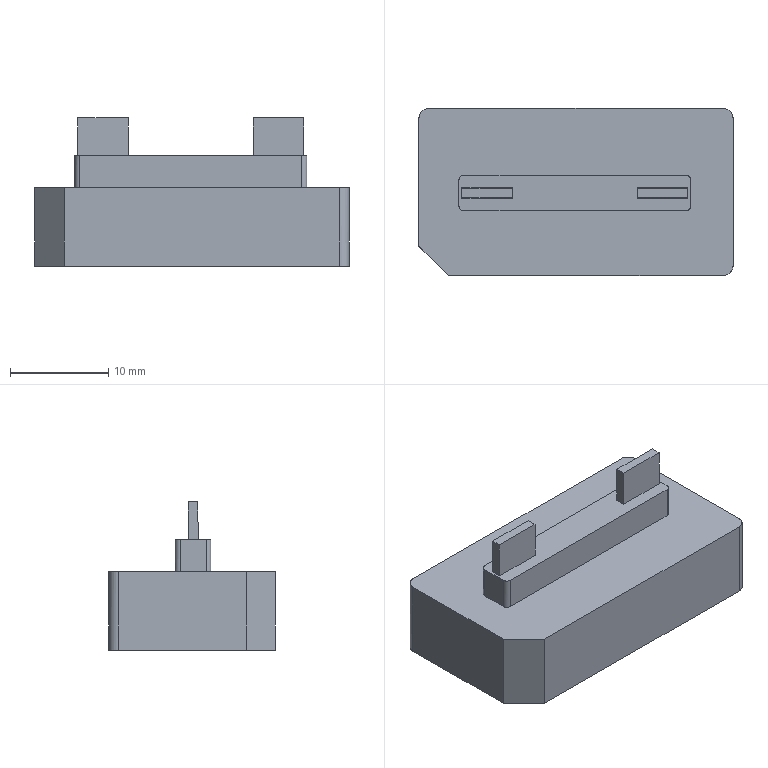NC program | PowerMill | posted by the shop | part box 32 x 17 x 15.109 mm
Lines 3996 to 5578 of 56729:
( TOOL ID   D3_1_1 )
( TOOL DIA. 3. TIP RAD 0 LENGTH 62.28 )
( Z = -7.28 )
T10 M6
T13
G91 G28 Z0
G0 G90 G54
M08
S18000 M3
X0 Y0 M8
G43 Z10.799 H10
X12.158 Y-2.407
Z.922
G1 Z-.278 F1200
X12.15 Y-2.364 F2000
X12.138 Y-2.322
X12.122 Y-2.282
X12.102 Y-2.242
X12.08 Y-2.205
X12.053 Y-2.17
X12.024 Y-2.137
X11.992 Y-2.108
X11.957 Y-2.081
X11.92 Y-2.058
X11.881 Y-2.038
X11.841 Y-2.022
X11.799 Y-2.009
X11.756 Y-2.
X11.712 Y-1.996
X11.669 Y-1.995
X11.625 Y-1.998
X11.615 Y-1.999
X11.542 Y-2.01
X11.471 Y-2.016
X11.402 Y-2.018
X11.333
X8.245
X6.298 Y-2.019
X6.211 Y-2.017
X6.129 Y-2.012
X6.053 Y-2.004
X5.981 Y-1.992
X5.913 Y-1.977
X5.847 Y-1.958
X5.775 Y-1.935
X5.704 Y-1.907
X5.635 Y-1.876
X5.568 Y-1.841
X5.503 Y-1.802
X5.439 Y-1.761
X5.379 Y-1.716
X5.321 Y-1.668
X5.266 Y-1.618
X5.214 Y-1.564
X5.164 Y-1.508
X5.117 Y-1.449
X5.073 Y-1.387
X5.033 Y-1.323
X4.996 Y-1.257
X4.962 Y-1.189
X4.932 Y-1.12
X4.906 Y-1.049
X4.884 Y-.978
X4.866 Y-.905
X4.851 Y-.831
X4.841 Y-.757
X4.834 Y-.683
X4.832 Y-.608
Y-.533
X4.831 Y.3
X4.832 Y.366
X4.834 Y.432
X4.839 Y.498
X4.846 Y.564
X4.856 Y.631
X4.87 Y.699
X4.888 Y.767
X4.91 Y.835
X4.935 Y.9
X4.962 Y.963
X4.992 Y1.026
X5.026 Y1.088
X5.063 Y1.149
X5.105 Y1.21
X5.152 Y1.269
X5.199 Y1.324
X5.25 Y1.378
X5.304 Y1.429
X5.361 Y1.478
X5.421 Y1.524
X5.484 Y1.566
X5.548 Y1.606
X5.615 Y1.642
X5.684 Y1.674
X5.751 Y1.702
X5.821 Y1.726
X5.894 Y1.747
X5.969 Y1.765
X6.034 Y1.777
X6.102 Y1.786
X6.176 Y1.792
X6.26 Y1.794
X6.36 Y1.795
X10.154 Y1.794
X11.397
X11.468 Y1.792
X11.539 Y1.786
X11.61 Y1.777
X11.681 Y1.763
X11.753 Y1.746
X11.825 Y1.724
X11.894 Y1.699
X11.963 Y1.671
X12.031 Y1.638
X12.097 Y1.602
X12.161 Y1.563
X12.223 Y1.52
X12.283 Y1.474
X12.34 Y1.425
X12.395 Y1.372
X12.446 Y1.317
X12.495 Y1.26
X12.541 Y1.2
X12.583 Y1.137
X12.621 Y1.075
X12.656 Y1.009
X12.688 Y.941
X12.716 Y.872
X12.74 Y.803
X12.757 Y.744
X12.772 Y.684
X12.784 Y.624
X12.794 Y.559
X12.802 Y.487
X12.807 Y.407
X12.808 Y.333
X12.809 Y.264
Y.2
X12.808 Y-.397
X12.807 Y-.6
X12.805 Y-.673
X12.799 Y-.747
X12.789 Y-.821
X12.775 Y-.894
X12.758 Y-.967
X12.736 Y-1.04
X12.71 Y-1.111
X12.681 Y-1.18
X12.649 Y-1.248
X12.612 Y-1.313
X12.573 Y-1.377
X12.529 Y-1.439
X12.483 Y-1.499
X12.434 Y-1.555
X12.382 Y-1.61
X12.326 Y-1.661
X12.269 Y-1.709
X12.209 Y-1.754
X12.146 Y-1.796
X12.081 Y-1.835
X12.014 Y-1.871
X11.946 Y-1.902
X11.875 Y-1.93
X11.804 Y-1.955
X11.731 Y-1.975
X11.657 Y-1.992
X11.615 Y-1.999
X11.545 Y-2.01
X11.474 Y-2.016
X11.403 Y-2.018 Z-.279
X11.332
X6.298 Y-2.019 Z-.286
X6.213 Y-2.017
X6.132 Y-2.012
X6.056 Y-2.004
X5.982 Y-1.992
X5.912 Y-1.977
X5.844 Y-1.958
X5.776 Y-1.935
X5.705 Y-1.908 Z-.287
X5.636 Y-1.876
X5.569 Y-1.842
X5.504 Y-1.803
X5.44 Y-1.762
X5.38 Y-1.717
X5.322 Y-1.669
X5.266 Y-1.618
X5.213 Y-1.564
X5.163 Y-1.508 Z-.288
X5.117 Y-1.449
X5.073 Y-1.387
X5.033 Y-1.324
X4.996 Y-1.258
X4.962 Y-1.19
X4.932 Y-1.12
X4.906 Y-1.049
X4.884 Y-.977
X4.866 Y-.905 Z-.289
X4.851 Y-.831
X4.841 Y-.757
X4.834 Y-.683
X4.832 Y-.609
Y-.535
Y.4 Z-.29
X4.835 Y.468
X4.841 Y.537 Z-.291
X4.851 Y.608
X4.865 Y.679
X4.884 Y.752
X4.906 Y.825
X4.933 Y.898
X4.962 Y.966
X4.995 Y1.033
X5.032 Y1.098
X5.072 Y1.162 Z-.292
X5.115 Y1.223
X5.163 Y1.283
X5.212 Y1.339
X5.264 Y1.392
X5.319 Y1.443
X5.377 Y1.491
X5.438 Y1.536
X5.501 Y1.578
X5.567 Y1.617
X5.631 Y1.65 Z-.293
X5.697 Y1.68
X5.767 Y1.708
X5.84 Y1.732
X5.903 Y1.751
X5.967 Y1.765
X6.035 Y1.777
X6.108 Y1.786
X6.187 Y1.792
X6.274 Y1.794 Z-.294
X6.373 Y1.795
X8.854 Z-.297
X10.122 Z-.299
X11.368 Y1.794 Z-.301
X11.442 Y1.793
X11.515 Y1.788
X11.588 Y1.78
X11.662 Y1.767
X11.734 Y1.751
X11.806 Y1.73
X11.878 Y1.706
X11.948 Y1.678 Z-.302
X12.016 Y1.646
X12.083 Y1.611
X12.148 Y1.572
X12.21 Y1.53
X12.27 Y1.484
X12.328 Y1.436
X12.383 Y1.384
X12.436 Y1.33
X12.485 Y1.273 Z-.303
X12.531 Y1.213
X12.574 Y1.151
X12.614 Y1.087
X12.65 Y1.022
X12.682 Y.955
X12.71 Y.887
X12.736 Y.814
X12.758 Y.741
X12.776 Y.669
X12.79 Y.597 Z-.304
X12.799 Y.525
X12.805 Y.454
X12.807 Y.384
X12.808 Y-.029
X12.807 Y-.6 Z-.305
X12.805 Y-.675
X12.799 Y-.749 Z-.306
X12.789 Y-.823
X12.775 Y-.897
X12.757 Y-.97
X12.735 Y-1.042
X12.71 Y-1.113
X12.68 Y-1.182
X12.647 Y-1.25
X12.611 Y-1.316
X12.571 Y-1.38
X12.528 Y-1.442 Z-.307
X12.481 Y-1.501
X12.432 Y-1.558
X12.379 Y-1.612
X12.324 Y-1.663
X12.266 Y-1.712
X12.206 Y-1.757
X12.143 Y-1.799
X12.078 Y-1.837
X12.012 Y-1.872 Z-.308
X11.943 Y-1.904
X11.873 Y-1.932
X11.802 Y-1.956
X11.729 Y-1.976
X11.655 Y-1.992
X11.615 Y-2.
X11.545 Y-2.01
X11.474 Y-2.016
X11.403 Y-2.019
X11.332 Z-.309
X7.573 Z-.314
X6.334 Y-2.02 Z-.316
X6.249 Y-2.019
X6.168 Y-2.015
X6.089 Y-2.008
X6.013 Y-1.997
X5.939 Y-1.983
X5.867 Y-1.965
X5.797 Y-1.943
X5.73 Y-1.918
X5.663 Y-1.89 Z-.317
X5.595 Y-1.856
X5.529 Y-1.819
X5.464 Y-1.778
X5.403 Y-1.735
X5.344 Y-1.688
X5.287 Y-1.639
X5.233 Y-1.586
X5.182 Y-1.531
X5.134 Y-1.473 Z-.318
X5.089 Y-1.412
X5.048 Y-1.349
X5.01 Y-1.284
X4.975 Y-1.217
X4.943 Y-1.149
X4.916 Y-1.078
X4.892 Y-1.007
X4.872 Y-.935
X4.856 Y-.861
X4.844 Y-.787 Z-.319
X4.836 Y-.713
X4.832 Y-.638
Y-.563
X4.831 Y.006 Z-.32
X4.832 Y.4
X4.835 Y.471
X4.841 Y.542
X4.852 Y.614 Z-.321
X4.866 Y.686
X4.885 Y.758
X4.908 Y.83
X4.935 Y.902
X4.965 Y.973
X4.998 Y1.039
X5.034 Y1.104
X5.074 Y1.166
X5.118 Y1.227 Z-.322
X5.165 Y1.286
X5.215 Y1.343
X5.269 Y1.397
X5.324 Y1.447
X5.382 Y1.495
X5.442 Y1.539
X5.505 Y1.581
X5.571 Y1.619
X5.639 Y1.654 Z-.323
X5.704 Y1.684
X5.771 Y1.71
X5.839 Y1.733
X5.91 Y1.752
X5.982 Y1.768
X6.057 Y1.78
X6.135 Y1.789
X6.217 Y1.794
X6.298 Y1.796
X7.812 Y1.795 Z-.326
X10.122 Z-.329
X11.397 Y1.794 Z-.331
X11.47 Y1.792
X11.543 Y1.786
X11.616 Y1.776
X11.689 Y1.762
X11.761 Y1.744
X11.833 Y1.722
X11.904 Y1.696
X11.974 Y1.666 Z-.332
X12.042 Y1.633
X12.108 Y1.596
X12.172 Y1.556
X12.234 Y1.513
X12.293 Y1.466
X12.349 Y1.418
X12.402 Y1.366
X12.453 Y1.31
X12.502 Y1.252
X12.547 Y1.191 Z-.333
X12.589 Y1.128
X12.627 Y1.064
X12.662 Y.998
X12.693 Y.931
X12.72 Y.863
X12.744 Y.79
X12.765 Y.717
X12.781 Y.644
X12.794 Y.572 Z-.334
X12.802 Y.501
X12.806 Y.432
X12.807 Y.364
X12.808 Y-.263 Z-.335
X12.807 Y-.6
X12.805 Y-.675
X12.799 Y-.75
X12.789 Y-.824 Z-.336
X12.775 Y-.898
X12.757 Y-.971
X12.735 Y-1.043
X12.709 Y-1.114
X12.68 Y-1.184
X12.647 Y-1.252
X12.61 Y-1.318
X12.57 Y-1.381
X12.527 Y-1.443
X12.481 Y-1.502 Z-.337
X12.431 Y-1.559
X12.379 Y-1.613
X12.323 Y-1.664
X12.265 Y-1.713
X12.205 Y-1.758
X12.142 Y-1.8
X12.077 Y-1.838
X12.01 Y-1.873
X11.942 Y-1.905 Z-.338
X11.872 Y-1.932
X11.8 Y-1.956
X11.727 Y-1.977
X11.654 Y-1.993
X11.615 Y-2.
X11.545 Y-2.01
X11.474 Y-2.017
X11.403 Y-2.019
X11.332
X7.573 Z-.344
X6.336 Y-2.02 Z-.346
X6.251
X6.169 Y-2.016
X6.09 Y-2.009
X6.014 Y-1.998
X5.94 Y-1.983
X5.868 Y-1.965
X5.799 Y-1.944
X5.731 Y-1.919
X5.664 Y-1.891
X5.596 Y-1.857 Z-.347
X5.529 Y-1.82
X5.465 Y-1.78
X5.404 Y-1.736
X5.344 Y-1.689
X5.288 Y-1.64
X5.234 Y-1.587
X5.183 Y-1.532
X5.135 Y-1.474
X5.09 Y-1.413 Z-.348
X5.048 Y-1.351
X5.01 Y-1.286
X4.975 Y-1.219
X4.944 Y-1.15
X4.916 Y-1.08
X4.892 Y-1.009
X4.872 Y-.936
X4.856 Y-.863
X4.844 Y-.789 Z-.349
X4.836 Y-.714
X4.832 Y-.64
X4.831 Y-.564
Y.007 Z-.35
X4.832 Y.4
X4.834 Y.471
X4.841 Y.542
X4.852 Y.614 Z-.351
X4.866 Y.686
X4.885 Y.758
X4.907 Y.83
X4.934 Y.902
X4.965 Y.973
X4.998 Y1.039
X5.034 Y1.104
X5.074 Y1.167
X5.118 Y1.228
X5.165 Y1.286 Z-.352
X5.215 Y1.343
X5.268 Y1.397
X5.323 Y1.448
X5.381 Y1.495
X5.442 Y1.54
X5.505 Y1.581
X5.57 Y1.619
X5.638 Y1.654
X5.704 Y1.684 Z-.353
X5.771 Y1.71
X5.839 Y1.733
X5.909 Y1.752
X5.982 Y1.768
X6.057 Y1.78
X6.135 Y1.789
X6.216 Y1.794
X6.298 Y1.796
X7.81 Y1.795 Z-.356
X10.122 Z-.359
X11.369 Y1.794 Z-.361
X11.442
X11.515 Y1.789
X11.589 Y1.78
X11.662 Y1.768
X11.734 Y1.751
X11.806 Y1.731
X11.878 Y1.706
X11.948 Y1.678
X12.016 Y1.646 Z-.362
X12.083 Y1.611
X12.148 Y1.572
X12.21 Y1.53
X12.271 Y1.485
X12.328 Y1.436
X12.383 Y1.385
X12.436 Y1.33
X12.485 Y1.273
X12.531 Y1.213
X12.574 Y1.151 Z-.363
X12.614 Y1.088
X12.65 Y1.022
X12.682 Y.955
X12.71 Y.887
X12.736 Y.814
X12.758 Y.742
X12.776 Y.669
X12.79 Y.597
X12.799 Y.525 Z-.364
X12.805 Y.454
X12.807 Y.384
X12.808 Y-.03
X12.807 Y-.6 Z-.365
X12.805 Y-.675
X12.799 Y-.749
X12.789 Y-.823
X12.775 Y-.897 Z-.366
X12.757 Y-.97
X12.736 Y-1.042
X12.71 Y-1.113
X12.681 Y-1.182
X12.648 Y-1.25
X12.611 Y-1.316
X12.571 Y-1.38
X12.528 Y-1.442
X12.482 Y-1.501 Z-.367
X12.432 Y-1.558
X12.38 Y-1.612
X12.324 Y-1.664
X12.267 Y-1.712
X12.206 Y-1.757
X12.144 Y-1.799
X12.079 Y-1.838
X12.012 Y-1.873
X11.943 Y-1.904
X11.873 Y-1.932 Z-.368
X11.802 Y-1.956
X11.729 Y-1.976
X11.656 Y-1.993
X11.615 Y-2.
X11.545 Y-2.01
X11.474 Y-2.017
X11.403 Y-2.019
X11.332
X7.573 Z-.374
X6.337 Y-2.02 Z-.375
X6.252 Z-.376
X6.17 Y-2.016
X6.091 Y-2.009
X6.015 Y-1.998
X5.941 Y-1.984
X5.869 Y-1.966
X5.8 Y-1.945
X5.732 Y-1.92
X5.665 Y-1.891
X5.597 Y-1.858 Z-.377
X5.531 Y-1.821
X5.466 Y-1.781
X5.405 Y-1.737
X5.345 Y-1.691
X5.289 Y-1.641
X5.235 Y-1.589
X5.184 Y-1.533
X5.136 Y-1.475
X5.091 Y-1.415
X5.049 Y-1.352 Z-.378
X5.01 Y-1.287
X4.975 Y-1.22
X4.944 Y-1.152
X4.916 Y-1.082
X4.893 Y-1.01
X4.873 Y-.938
X4.856 Y-.865
X4.844 Y-.791
X4.836 Y-.716 Z-.379
X4.832 Y-.641
X4.831 Y-.566
X4.83 Y.008 Z-.38
X4.832 Y.4
X4.834 Y.471
X4.841 Y.542
X4.851 Y.614
X4.866 Y.686 Z-.381
X4.884 Y.759
X4.907 Y.831
X4.934 Y.902
X4.965 Y.973
X4.997 Y1.039
X5.034 Y1.104
X5.074 Y1.167
X5.117 Y1.228
X5.164 Y1.287
X5.215 Y1.343 Z-.382
X5.268 Y1.397
X5.323 Y1.448
X5.381 Y1.495
X5.442 Y1.54
X5.505 Y1.581
X5.57 Y1.619
X5.638 Y1.654
X5.703 Y1.684
X5.77 Y1.71 Z-.383
X5.839 Y1.733
X5.909 Y1.752
X5.981 Y1.768
X6.056 Y1.78
X6.134 Y1.789
X6.216 Y1.795
X6.298 Y1.796
X7.808 Y1.795 Z-.385
X10.122 Z-.389
X11.369 Z-.39
X11.442 Y1.794 Z-.391
X11.515 Y1.789
X11.588 Y1.781
X11.662 Y1.768
X11.734 Y1.752
X11.806 Y1.731
X11.878 Y1.707
X11.948 Y1.678
X12.016 Y1.647
X12.083 Y1.611 Z-.392
X12.148 Y1.573
X12.21 Y1.53
X12.271 Y1.485
X12.328 Y1.436
X12.383 Y1.385
X12.436 Y1.33
X12.485 Y1.273
X12.531 Y1.214
X12.574 Y1.152 Z-.393
X12.614 Y1.088
X12.65 Y1.023
X12.682 Y.956
X12.71 Y.887
X12.736 Y.815
X12.758 Y.742
X12.776 Y.67
X12.79 Y.597
X12.799 Y.526
X12.805 Y.455 Z-.394
X12.807 Y.384
X12.808 Y-.03
X12.807 Y-.6 Z-.395
X12.805 Y-.675
X12.799 Y-.749
X12.789 Y-.824
X12.775 Y-.897
X12.757 Y-.97 Z-.396
X12.736 Y-1.042
X12.71 Y-1.113
X12.681 Y-1.183
X12.648 Y-1.25
X12.611 Y-1.316
X12.571 Y-1.381
X12.528 Y-1.442
X12.482 Y-1.502
X12.432 Y-1.558 Z-.397
X12.38 Y-1.613
X12.325 Y-1.664
X12.267 Y-1.712
X12.206 Y-1.757
X12.144 Y-1.799
X12.079 Y-1.838
X12.012 Y-1.873
X11.943 Y-1.905
X11.873 Y-1.932 Z-.398
X11.802 Y-1.956
X11.729 Y-1.977
X11.656 Y-1.993
X11.615 Y-2.
X11.545 Y-2.011
X11.474 Y-2.017
X11.403 Y-2.019
X11.332 Y-2.02
X7.573 Z-.404
X6.338 Z-.405
X6.253
X6.171 Y-2.017 Z-.406
X6.092 Y-2.009
X6.016 Y-1.999
X5.942 Y-1.984
X5.87 Y-1.967
X5.801 Y-1.945
X5.733 Y-1.921
X5.666 Y-1.892
X5.598 Y-1.859
X5.531 Y-1.822 Z-.407
X5.467 Y-1.782
X5.405 Y-1.738
X5.346 Y-1.692
X5.289 Y-1.642
X5.236 Y-1.59
X5.184 Y-1.534
X5.136 Y-1.477
X5.091 Y-1.416
X5.049 Y-1.354 Z-.408
X5.011 Y-1.289
X4.976 Y-1.222
X4.944 Y-1.153
X4.917 Y-1.083
X4.893 Y-1.012
X4.873 Y-.939
X4.856 Y-.866
X4.844 Y-.792
X4.836 Y-.718
X4.831 Y-.643 Z-.409
Y-.568
X4.83 Y.008
X4.831 Y.4 Z-.41
X4.834 Y.471
X4.84 Y.542
X4.851 Y.614
X4.866 Y.687
X4.884 Y.759 Z-.411
X4.907 Y.831
X4.934 Y.902
X4.964 Y.973
X4.997 Y1.039
X5.034 Y1.104
X5.074 Y1.167
X5.117 Y1.228
X5.164 Y1.287
X5.214 Y1.343 Z-.412
X5.268 Y1.398
X5.323 Y1.448
X5.38 Y1.495
X5.441 Y1.54
X5.504 Y1.581
X5.569 Y1.619
X5.637 Y1.654
X5.702 Y1.684
X5.769 Y1.71
X5.837 Y1.733 Z-.413
X5.907 Y1.752
X5.98 Y1.768
X6.055 Y1.781
X6.133 Y1.789
X6.214 Y1.795
X6.298 Y1.796
X7.808 Z-.415
X10.122 Z-.419
X11.253 Y1.795 Z-.42
X11.397
X11.471 Y1.793 Z-.421
X11.544 Y1.786
X11.618 Y1.776
X11.691 Y1.762
X11.763 Y1.744
X11.835 Y1.722
X11.905 Y1.697
X11.975 Y1.667
X12.042 Y1.634
X12.109 Y1.597 Z-.422
X12.173 Y1.557
X12.234 Y1.513
X12.294 Y1.467
X12.35 Y1.417
X12.404 Y1.364
X12.455 Y1.309
X12.504 Y1.25
X12.549 Y1.19
X12.59 Y1.127
X12.629 Y1.062 Z-.423
X12.664 Y.995
X12.695 Y.926
X12.723 Y.856
X12.746 Y.785
X12.766 Y.713
X12.782 Y.641
X12.794 Y.568
X12.802 Y.495
X12.806 Y.422 Z-.424
Y.349
X12.808 Y-.064
X12.807 Y-.6 Z-.425
X12.805 Y-.675
X12.799 Y-.75
X12.789 Y-.825
X12.775 Y-.899
X12.757 Y-.972 Z-.426
X12.735 Y-1.044
X12.709 Y-1.115
X12.68 Y-1.184
X12.647 Y-1.252
X12.611 Y-1.318
X12.571 Y-1.382
X12.527 Y-1.443
X12.481 Y-1.503
X12.431 Y-1.559
X12.379 Y-1.614 Z-.427
X12.324 Y-1.665
X12.266 Y-1.713
X12.205 Y-1.758
X12.143 Y-1.8
X12.078 Y-1.839
X12.011 Y-1.874
X11.942 Y-1.905
X11.872 Y-1.933
X11.801 Y-1.957 Z-.428
X11.728 Y-1.977
X11.655 Y-1.994
X11.615 Y-2.001
X11.545 Y-2.011
X11.474 Y-2.017
X11.404 Y-2.02
X11.333
X7.573 Z-.434
X6.34 Y-2.021 Z-.435
X6.255 Y-2.02
X6.173 Y-2.017 Z-.436
X6.094 Y-2.01
X6.017 Y-1.999
X5.943 Y-1.985
X5.871 Y-1.967
X5.802 Y-1.946
X5.734 Y-1.921
X5.667 Y-1.893
X5.599 Y-1.86
X5.532 Y-1.823
X5.468 Y-1.783 Z-.437
X5.406 Y-1.739
X5.347 Y-1.693
X5.29 Y-1.643
X5.236 Y-1.591
X5.185 Y-1.536
X5.137 Y-1.478
X5.092 Y-1.418
X5.05 Y-1.355
X5.011 Y-1.29 Z-.438
X4.976 Y-1.223
X4.945 Y-1.155
X4.917 Y-1.085
X4.893 Y-1.014
X4.873 Y-.941
X4.856 Y-.868
X4.844 Y-.794
X4.836 Y-.719
X4.831 Y-.644
X4.83 Y-.569 Z-.439
Y.009
X4.831 Y.4 Z-.44
X4.834 Y.471
X4.84 Y.543
X4.851 Y.615
X4.865 Y.687
X4.884 Y.759
X4.907 Y.831 Z-.441
X4.933 Y.902
X4.964 Y.973
X4.997 Y1.04
X5.033 Y1.104
X5.073 Y1.167
X5.117 Y1.228
X5.164 Y1.287
X5.214 Y1.344
X5.267 Y1.398 Z-.442
X5.322 Y1.448
X5.38 Y1.495
X5.44 Y1.54
X5.503 Y1.581
X5.569 Y1.619
X5.636 Y1.654
X5.702 Y1.684
X5.769 Y1.71
X5.837 Y1.733 Z-.443
X5.907 Y1.752
X5.979 Y1.768
X6.054 Y1.781
X6.132 Y1.79
X6.213 Y1.795
X6.298 Y1.797
X7.806 Y1.796 Z-.445
X10.122 Z-.449
X11.368 Y1.795 Z-.45
X11.442 Y1.794
X11.515 Y1.79 Z-.451
X11.588 Y1.781
X11.661 Y1.769
X11.734 Y1.752
X11.806 Y1.732
X11.877 Y1.707
X11.948 Y1.679
X12.016 Y1.647
X12.083 Y1.612
X12.147 Y1.573 Z-.452
X12.21 Y1.531
X12.27 Y1.486
X12.328 Y1.437
X12.383 Y1.386
X12.435 Y1.331
X12.485 Y1.274
X12.531 Y1.215
X12.574 Y1.153
X12.614 Y1.089
X12.65 Y1.023 Z-.453
X12.682 Y.956
X12.711 Y.887
X12.737 Y.815
X12.758 Y.742
X12.776 Y.67
X12.79 Y.598
X12.799 Y.526
X12.805 Y.454
X12.807 Y.384 Z-.454
X12.808 Y-.026
X12.807 Y-.6 Z-.455
X12.805 Y-.675
X12.799 Y-.749
X12.789 Y-.824
X12.775 Y-.897
X12.757 Y-.97
X12.736 Y-1.042 Z-.456
X12.71 Y-1.113
X12.681 Y-1.183
X12.648 Y-1.251
X12.611 Y-1.317
X12.571 Y-1.381
X12.528 Y-1.443
X12.482 Y-1.502
X12.433 Y-1.559
X12.38 Y-1.613 Z-.457
X12.325 Y-1.664
X12.267 Y-1.712
X12.207 Y-1.757
X12.144 Y-1.799
X12.079 Y-1.838
X12.013 Y-1.873
X11.944 Y-1.905
X11.874 Y-1.933
X11.803 Y-1.957
X11.73 Y-1.977 Z-.458
X11.657 Y-1.993
X11.615 Y-2.001
X11.545 Y-2.011
X11.475 Y-2.018
X11.404 Y-2.02
X11.333
X7.573 Z-.463
X6.341 Y-2.021 Z-.465
X6.256
X6.174 Y-2.017
X6.095 Y-2.01 Z-.466
X6.018 Y-2.
X5.944 Y-1.986
X5.873 Y-1.968
X5.803 Y-1.947
X5.735 Y-1.922
X5.668 Y-1.894
X5.6 Y-1.861
X5.533 Y-1.824
X5.469 Y-1.784 Z-.467
X5.407 Y-1.74
X5.348 Y-1.694
X5.291 Y-1.645
X5.237 Y-1.592
X5.186 Y-1.537
X5.137 Y-1.479
X5.092 Y-1.419
X5.05 Y-1.357
X5.012 Y-1.292
X4.977 Y-1.225 Z-.468
X4.945 Y-1.156
X4.917 Y-1.086
X4.893 Y-1.015
X4.873 Y-.943
X4.856 Y-.869
X4.844 Y-.795
X4.836 Y-.721
X4.831 Y-.646
X4.83 Y-.571 Z-.469
Y.009
X4.831 Y.4 Z-.47
X4.833 Y.471
X4.84 Y.543
X4.85 Y.615
X4.865 Y.687
X4.884 Y.759
X4.906 Y.831 Z-.471
X4.933 Y.903
X4.964 Y.973
X4.997 Y1.04
X5.033 Y1.104
X5.073 Y1.167
X5.116 Y1.228
X5.163 Y1.287
X5.214 Y1.344
X5.267 Y1.398
X5.322 Y1.448 Z-.472
X5.38 Y1.496
X5.44 Y1.54
X5.503 Y1.581
X5.568 Y1.62
X5.636 Y1.655
X5.702 Y1.684
X5.768 Y1.711
X5.836 Y1.733
X5.906 Y1.753 Z-.473
X5.979 Y1.769
X6.054 Y1.781
X6.132 Y1.79
X6.213 Y1.795
X6.298 Y1.797
X7.804 Y1.796 Z-.475
X10.122 Z-.478
X11.368 Y1.795 Z-.48
X11.442
X11.515 Y1.79
X11.588 Y1.781 Z-.481
X11.661 Y1.769
X11.734 Y1.752
X11.806 Y1.732
X11.877 Y1.708
X11.948 Y1.679
X12.016 Y1.648
X12.083 Y1.612
X12.147 Y1.574
X12.21 Y1.531 Z-.482
X12.27 Y1.486
X12.328 Y1.437
X12.383 Y1.386
X12.435 Y1.332
X12.485 Y1.274
X12.531 Y1.215
X12.574 Y1.153
X12.614 Y1.089
X12.65 Y1.023
X12.682 Y.956 Z-.483
X12.711 Y.887
X12.737 Y.815
X12.758 Y.743
X12.776 Y.67
X12.79 Y.598
X12.799 Y.526
X12.805 Y.455
X12.807 Y.384
X12.808 Y-.026 Z-.484
X12.807 Y-.6 Z-.485
X12.805 Y-.675
X12.799 Y-.749
X12.789 Y-.824
X12.775 Y-.897
X12.757 Y-.97
X12.736 Y-1.042
X12.71 Y-1.113 Z-.486
X12.681 Y-1.183
X12.648 Y-1.251
X12.611 Y-1.317
X12.571 Y-1.381
X12.528 Y-1.443
X12.482 Y-1.502
X12.433 Y-1.559
X12.38 Y-1.613
X12.325 Y-1.664 Z-.487
X12.267 Y-1.712
X12.207 Y-1.758
X12.144 Y-1.8
X12.08 Y-1.838
X12.013 Y-1.873
X11.944 Y-1.905
X11.874 Y-1.933
X11.803 Y-1.957
X11.73 Y-1.977
X11.657 Y-1.994 Z-.488
X11.615 Y-2.001
X11.545 Y-2.011
X11.475 Y-2.018
X11.404 Y-2.02
X11.333
X7.573 Y-2.021 Z-.493
X6.325 Z-.495
X6.24
X6.159 Y-2.016
X6.08 Y-2.009
X6.004 Y-1.998 Z-.496
X5.931 Y-1.983
X5.859 Y-1.965
X5.79 Y-1.943
X5.722 Y-1.917
X5.656 Y-1.889
X5.588 Y-1.855
X5.522 Y-1.817
X5.458 Y-1.777
X5.396 Y-1.733 Z-.497
X5.337 Y-1.686
X5.281 Y-1.636
X5.227 Y-1.583
X5.177 Y-1.527
X5.129 Y-1.469
X5.084 Y-1.409
X5.043 Y-1.346
X5.005 Y-1.28
X4.97 Y-1.213 Z-.498
X4.94 Y-1.145
X4.912 Y-1.074
X4.889 Y-1.003
X4.869 Y-.93
X4.854 Y-.857
X4.842 Y-.783
X4.834 Y-.708
X4.83 Y-.633
Y-.558
X4.829 Y.017 Z-.499
X4.831 Y.4 Z-.5
X4.833 Y.471
X4.84 Y.543
X4.85 Y.615
X4.865 Y.687
X4.883 Y.759
X4.906 Y.831
X4.933 Y.903 Z-.501
X4.963 Y.973
X4.996 Y1.04
X5.033 Y1.105
X5.073 Y1.168
X5.117 Y1.229
X5.164 Y1.288
X5.214 Y1.345
X5.267 Y1.398
X5.322 Y1.449 Z-.502
X5.381 Y1.497
X5.441 Y1.541
X5.505 Y1.583
X5.57 Y1.621
X5.638 Y1.656
X5.703 Y1.686
X5.77 Y1.712
X5.838 Y1.734
X5.909 Y1.754
X5.981 Y1.769 Z-.503
X6.056 Y1.782
X6.134 Y1.79
X6.216 Y1.796
X6.298 Y1.797
X7.797 Y1.796 Z-.505
X10.122 Z-.508
X11.368 Z-.51
X11.442 Y1.795
X11.515 Y1.79
X11.588 Y1.782
X11.661 Y1.769 Z-.511
X11.734 Y1.753
X11.806 Y1.732
X11.877 Y1.708
X11.948 Y1.68
X12.016 Y1.648
X12.083 Y1.613
X12.147 Y1.574
X12.21 Y1.532
X12.27 Y1.486 Z-.512
X12.328 Y1.438
X12.383 Y1.386
X12.435 Y1.332
X12.485 Y1.275
X12.531 Y1.215
X12.574 Y1.153
X12.614 Y1.089
X12.65 Y1.024
X12.682 Y.956 Z-.513
X12.711 Y.888
X12.737 Y.815
X12.758 Y.743
X12.776 Y.67
X12.79 Y.598
X12.799 Y.526
X12.805 Y.455
X12.807 Y.384
X12.808 Y-.03 Z-.514
X12.807 Y-.6 Z-.515
X12.805 Y-.675
X12.799 Y-.75
X12.789 Y-.824
X12.775 Y-.898
X12.757 Y-.971
X12.736 Y-1.043
X12.71 Y-1.114
X12.681 Y-1.183 Z-.516
X12.648 Y-1.251
X12.611 Y-1.317
X12.572 Y-1.381
X12.528 Y-1.443
X12.482 Y-1.502
X12.433 Y-1.559
X12.38 Y-1.613
X12.325 Y-1.664
X12.268 Y-1.712 Z-.517
X12.207 Y-1.758
X12.145 Y-1.8
X12.08 Y-1.838
X12.013 Y-1.874
X11.945 Y-1.905
X11.875 Y-1.933
X11.803 Y-1.957
X11.731 Y-1.977
X11.658 Y-1.994 Z-.518
X11.616 Y-2.001
X11.545 Y-2.012
X11.475 Y-2.018
X11.404 Y-2.021
X11.333
X7.573 Z-.523
X6.329 Y-2.022 Z-.525
X6.244 Y-2.021
X6.163 Y-2.017
X6.084 Y-2.01
X6.008 Y-1.999 Z-.526
X5.934 Y-1.984
X5.863 Y-1.966
X5.793 Y-1.944
X5.725 Y-1.919
X5.659 Y-1.89
X5.591 Y-1.857
X5.525 Y-1.82
X5.461 Y-1.779
X5.399 Y-1.735
X5.34 Y-1.688 Z-.527
X5.283 Y-1.638
X5.229 Y-1.586
X5.179 Y-1.53
X5.131 Y-1.472
X5.086 Y-1.412
X5.045 Y-1.349
X5.006 Y-1.284
X4.972 Y-1.217
X4.941 Y-1.148 Z-.528
X4.913 Y-1.078
X4.89 Y-1.007
X4.87 Y-.934
X4.854 Y-.861
X4.842 Y-.786
X4.834 Y-.712
X4.83 Y-.637
Y-.561
X4.829 Y.127 Z-.529
X4.828 Y.294 Z-.53
X4.829 Y.364
X4.831 Y.438
X4.837 Y.514
X4.846 Y.587
X4.858 Y.654
X4.872 Y.719
X4.89 Y.782
X4.911 Y.845
X4.937 Y.916
X4.968 Y.984 Z-.531
X5.002 Y1.051
X5.039 Y1.117
X5.08 Y1.18
X5.125 Y1.241
X5.172 Y1.299
X5.223 Y1.355
X5.276 Y1.408
X5.332 Y1.458
X5.391 Y1.505 Z-.532
X5.452 Y1.549
X5.516 Y1.59
X5.582 Y1.628
X5.65 Y1.662
X5.719 Y1.693
X5.786 Y1.718
X5.854 Y1.739
X5.924 Y1.758
X5.995 Y1.772 Z-.533
X6.07 Y1.784
X6.148 Y1.792
X6.231 Y1.796
X6.317 Y1.797
X7.883 Z-.535
X10.122 Z-.538
X11.368 Y1.796 Z-.54
X11.442 Y1.795
X11.515 Y1.791
X11.588 Y1.782
X11.661 Y1.769 Z-.541
X11.734 Y1.753
X11.806 Y1.732
X11.877 Y1.708
X11.948 Y1.68
X12.016 Y1.648
X12.083 Y1.613
X12.147 Y1.574
X12.21 Y1.532
X12.27 Y1.486
X12.328 Y1.438 Z-.542
X12.383 Y1.386
X12.435 Y1.332
X12.485 Y1.275
X12.531 Y1.215
X12.574 Y1.154
X12.613 Y1.09
X12.649 Y1.025
X12.681 Y.958
X12.71 Y.889 Z-.543
X12.736 Y.816
X12.758 Y.743
X12.776 Y.67
X12.79 Y.597
X12.8 Y.525
X12.806 Y.454
X12.808 Y.383
X12.809 Y.06 Z-.544
X12.808 Y-.375
X12.807 Y-.6 Z-.545
X12.805 Y-.675
X12.799 Y-.75
X12.789 Y-.825
X12.775 Y-.899
X12.757 Y-.972
X12.735 Y-1.044
X12.71 Y-1.115
X12.68 Y-1.184 Z-.546
X12.647 Y-1.252
X12.611 Y-1.318
X12.571 Y-1.382
X12.528 Y-1.444
X12.481 Y-1.503
X12.432 Y-1.56
X12.38 Y-1.614
X12.325 Y-1.665
X12.267 Y-1.713
X12.207 Y-1.758 Z-.547
X12.144 Y-1.8
X12.079 Y-1.839
X12.012 Y-1.874
X11.944 Y-1.906
X11.874 Y-1.934
X11.802 Y-1.958
X11.73 Y-1.978
X11.657 Y-1.994
X11.616 Y-2.002 Z-.548
X11.545 Y-2.012
X11.475 Y-2.018
X11.404 Y-2.021
X11.333
X7.573 Z-.553
X6.364 Y-2.022 Z-.555
X6.279
X6.196 Y-2.019
X6.116 Y-2.013
X6.039 Y-2.004
X5.964 Y-1.99 Z-.556
X5.891 Y-1.974
X5.82 Y-1.953
X5.751 Y-1.93
X5.684 Y-1.902
X5.618 Y-1.871
X5.551 Y-1.836
X5.486 Y-1.796
X5.424 Y-1.754
X5.364 Y-1.708
X5.306 Y-1.66 Z-.557
X5.251 Y-1.608
X5.199 Y-1.554
X5.15 Y-1.496
X5.104 Y-1.437
X5.061 Y-1.375
X5.021 Y-1.311
X4.985 Y-1.245
X4.953 Y-1.177
X4.924 Y-1.107 Z-.558
X4.899 Y-1.036
X4.877 Y-.964
X4.86 Y-.89
X4.846 Y-.816
X4.837 Y-.742
X4.831 Y-.667
X4.829 Y-.591
Y.022 Z-.559
X4.83 Y.401 Z-.56
X4.833 Y.472
X4.839 Y.543
X4.85 Y.615
X4.864 Y.688
X4.883 Y.76
X4.906 Y.832
X4.932 Y.903
X4.962 Y.972
X4.995 Y1.04 Z-.561
X5.032 Y1.105
X5.073 Y1.169
X5.117 Y1.23
X5.164 Y1.289
X5.214 Y1.346
X5.267 Y1.399
X5.322 Y1.45
X5.381 Y1.498
X5.442 Y1.542 Z-.562
X5.505 Y1.584
X5.57 Y1.622
X5.638 Y1.657
X5.707 Y1.688
X5.774 Y1.714
X5.841 Y1.736
X5.91 Y1.755
X5.982 Y1.77
X6.056 Y1.782 Z-.563
X6.134 Y1.791
X6.215 Y1.796
X6.298 Y1.798
X7.861 Y1.797 Z-.565
X10.122 Z-.568
X11.368 Y1.796 Z-.57
X11.442 Y1.795
X11.515 Y1.791
X11.588 Y1.782
X11.661 Y1.77
X11.734 Y1.753 Z-.571
X11.806 Y1.733
X11.877 Y1.708
X11.948 Y1.68
X12.016 Y1.648
X12.083 Y1.613
X12.147 Y1.574
X12.21 Y1.532
X12.27 Y1.487
X12.328 Y1.438 Z-.572
X12.383 Y1.387
X12.435 Y1.332
X12.485 Y1.275
X12.531 Y1.216
X12.574 Y1.154
X12.613 Y1.09
X12.649 Y1.025
X12.681 Y.958
X12.71 Y.889
X12.736 Y.816 Z-.573
X12.758 Y.743
X12.776 Y.67
X12.79 Y.598
X12.8 Y.525
X12.806 Y.454
X12.808 Y.383
X12.809 Y.059 Z-.574
X12.808 Y-.379
X12.807 Y-.6 Z-.575
X12.805 Y-.675
X12.799 Y-.75
X12.789 Y-.825
X12.775 Y-.899
X12.757 Y-.972
X12.735 Y-1.044
X12.71 Y-1.115
X12.681 Y-1.184
X12.648 Y-1.252 Z-.576
X12.611 Y-1.318
X12.571 Y-1.382
X12.528 Y-1.444
X12.482 Y-1.503
X12.432 Y-1.56
X12.38 Y-1.614
X12.325 Y-1.665
X12.267 Y-1.713
X12.207 Y-1.759 Z-.577
X12.144 Y-1.801
X12.079 Y-1.839
X12.012 Y-1.874
X11.944 Y-1.906
X11.874 Y-1.934
X11.803 Y-1.958
X11.73 Y-1.978
X11.657 Y-1.994
X11.616 Y-2.002
X11.545 Y-2.012 Z-.578
X11.475 Y-2.019
X11.404 Y-2.021
X11.333
X7.573 Z-.583
X6.366 Y-2.022 Z-.585
X6.281
X6.198 Y-2.02
X6.118 Y-2.014
X6.04 Y-2.004
X5.965 Y-1.991
X5.892 Y-1.974 Z-.586
X5.822 Y-1.954
X5.753 Y-1.93
X5.686 Y-1.903
X5.62 Y-1.872
X5.553 Y-1.837
X5.488 Y-1.798
X5.425 Y-1.755
X5.365 Y-1.71
X5.307 Y-1.661
X5.252 Y-1.61 Z-.587
X5.2 Y-1.555
X5.151 Y-1.498
X5.105 Y-1.439
X5.062 Y-1.377
X5.022 Y-1.313
X4.986 Y-1.247
X4.953 Y-1.179
X4.924 Y-1.109
X4.899 Y-1.038 Z-.588
X4.878 Y-.966
X4.86 Y-.893
X4.846 Y-.819
X4.837 Y-.745
X4.831 Y-.67
X4.829 Y-.595
X4.828 Y-.006 Z-.589
X4.83 Y.382 Z-.59
X4.831 Y.453
X4.837 Y.524
X4.846 Y.596
X4.86 Y.669
X4.877 Y.741
X4.899 Y.813
X4.924 Y.884
X4.954 Y.955
X4.986 Y1.022 Z-.591
X5.022 Y1.088
X5.061 Y1.152
X5.103 Y1.213
X5.149 Y1.273
X5.199 Y1.33
X5.251 Y1.384
X5.306 Y1.436
X5.363 Y1.485
X5.424 Y1.53
X5.486 Y1.573 Z-.592
X5.551 Y1.612
X5.618 Y1.647
X5.687 Y1.68
X5.754 Y1.707
X5.821 Y1.73
X5.891 Y1.75
X5.963 Y1.767
X6.037 Y1.78
X6.115 Y1.789 Z-.593
X6.195 Y1.796
X6.28 Y1.798
X6.368
X7.858 Y1.797 Z-.595
X10.122 Z-.598
X11.368 Y1.796 Z-.6
X11.442
X11.515 Y1.791
X11.588 Y1.783
X11.661 Y1.77
X11.734 Y1.753
X11.806 Y1.733 Z-.601
X11.877 Y1.709
X11.948 Y1.68
X12.016 Y1.649
X12.083 Y1.613
X12.147 Y1.575
X12.21 Y1.532
X12.27 Y1.487
X12.328 Y1.438
X12.383 Y1.387 Z-.602
X12.435 Y1.333
X12.485 Y1.275
X12.531 Y1.216
X12.574 Y1.154
X12.613 Y1.091
X12.649 Y1.025
X12.681 Y.958
X12.71 Y.889
X12.736 Y.816
X12.758 Y.743 Z-.603
X12.776 Y.67
X12.79 Y.598
X12.8 Y.526
X12.806 Y.454